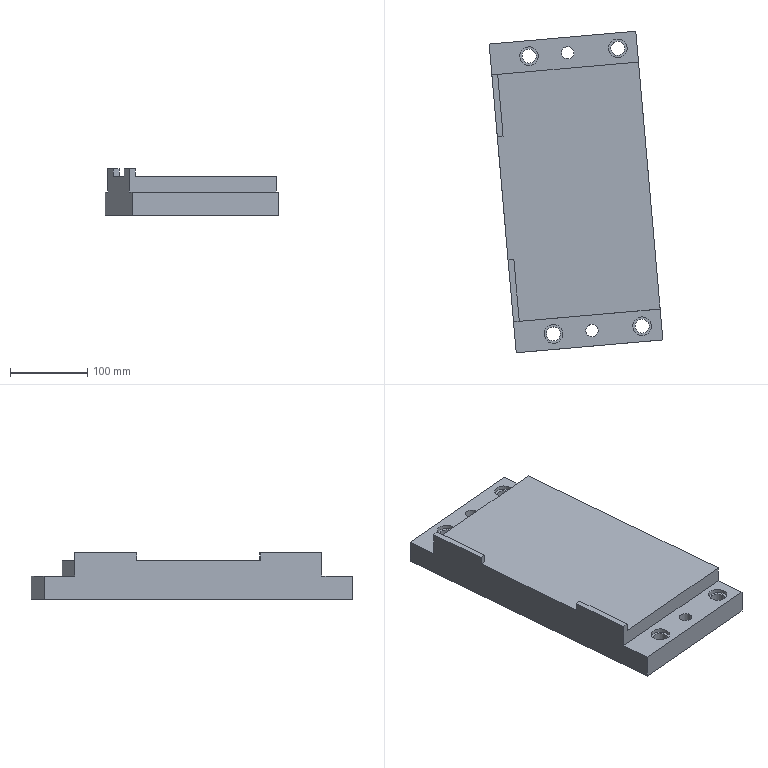Part | NX | features solid 2 | 1 solid | 35 faces | box 224.139 x 415.037 x 60 mm | volume 3448776 mm3 | plane 23 | cylinder 12 | commonest cylinder face diameters 18 x4 24 x4 16 x2 33.267 x2
STEP:
#1=CARTESIAN_POINT('',(824.667,699.536,-260.));
#2=VERTEX_POINT('',#1);
#3=CARTESIAN_POINT('',(831.64,619.841,-260.));
#4=VERTEX_POINT('',#3);
#5=CARTESIAN_POINT('',(824.667,699.536,-260.));
#6=DIRECTION('',(0.08716,-0.9962,0.));
#7=VECTOR('',#6,1000.);
#8=LINE('',#5,#7);
#9=EDGE_CURVE('',#2,#4,#8,.T.);
#10=ORIENTED_EDGE('',*,*,#9,.F.);
#11=CARTESIAN_POINT('',(817.198,698.883,-260.));
#12=VERTEX_POINT('',#11);
#13=CARTESIAN_POINT('',(824.667,699.536,-260.));
#14=DIRECTION('',(-0.9962,-0.08716,0.));
#15=VECTOR('',#14,1000.);
#16=LINE('',#13,#15);
#17=EDGE_CURVE('',#2,#12,#16,.T.);
#18=ORIENTED_EDGE('',*,*,#17,.T.);
#19=CARTESIAN_POINT('',(824.17,619.187,-260.));
#20=VERTEX_POINT('',#19);
#21=CARTESIAN_POINT('',(817.198,698.883,-260.));
#22=DIRECTION('',(0.08716,-0.9962,0.));
#23=VECTOR('',#22,1000.);
#24=LINE('',#21,#23);
#25=EDGE_CURVE('',#12,#20,#24,.T.);
#26=ORIENTED_EDGE('',*,*,#25,.T.);
#27=CARTESIAN_POINT('',(831.64,619.841,-260.));
#28=DIRECTION('',(-0.9962,-0.08716,0.));
#29=VECTOR('',#28,1000.);
#30=LINE('',#27,#29);
#31=EDGE_CURVE('',#4,#20,#30,.T.);
#32=ORIENTED_EDGE('',*,*,#31,.F.);
#33=EDGE_LOOP('',(#10,#18,#26,#32));
#34=FACE_BOUND('',#33,.T.);
#35=CARTESIAN_POINT('',(824.667,699.536,-260.));
#36=DIRECTION('',(0.,0.,-1.));
#37=DIRECTION('',(0.9962,0.08716,0.));
#38=AXIS2_PLACEMENT_3D('',#35,#36,#37);
#39=PLANE('',#38);
#40=ADVANCED_FACE('',(#34),#39,.F.);
#41=CARTESIAN_POINT('',(824.667,699.536,-270.));
#42=VERTEX_POINT('',#41);
#43=CARTESIAN_POINT('',(831.64,619.841,-270.));
#44=VERTEX_POINT('',#43);
#45=CARTESIAN_POINT('',(824.667,699.536,-270.));
#46=DIRECTION('',(0.08716,-0.9962,0.));
#47=VECTOR('',#46,1000.);
#48=LINE('',#45,#47);
#49=EDGE_CURVE('',#42,#44,#48,.T.);
#50=ORIENTED_EDGE('',*,*,#49,.F.);
#51=CARTESIAN_POINT('',(824.667,699.536,-270.));
#52=DIRECTION('',(0.,0.,1.));
#53=VECTOR('',#52,1000.);
#54=LINE('',#51,#53);
#55=EDGE_CURVE('',#42,#2,#54,.T.);
#56=ORIENTED_EDGE('',*,*,#55,.T.);
#57=ORIENTED_EDGE('',*,*,#9,.T.);
#58=CARTESIAN_POINT('',(831.64,619.841,-270.));
#59=DIRECTION('',(0.,0.,1.));
#60=VECTOR('',#59,1000.);
#61=LINE('',#58,#60);
#62=EDGE_CURVE('',#44,#4,#61,.T.);
#63=ORIENTED_EDGE('',*,*,#62,.F.);
#64=EDGE_LOOP('',(#50,#56,#57,#63));
#65=FACE_BOUND('',#64,.T.);
#66=CARTESIAN_POINT('',(824.667,699.536,-270.));
#67=DIRECTION('',(-0.9962,-0.08716,0.));
#68=DIRECTION('',(0.,0.,-1.));
#69=AXIS2_PLACEMENT_3D('',#66,#67,#68);
#70=PLANE('',#69);
#71=ADVANCED_FACE('',(#65),#70,.F.);
#72=CARTESIAN_POINT('',(1006.475,715.443,-290.));
#73=VERTEX_POINT('',#72);
#74=CARTESIAN_POINT('',(817.198,698.883,-290.));
#75=VERTEX_POINT('',#74);
#76=CARTESIAN_POINT('',(1006.475,715.443,-290.));
#77=DIRECTION('',(0.9962,0.08716,0.));
#78=VECTOR('',#77,1000.);
#79=LINE('',#76,#78);
#80=EDGE_CURVE('',#73,#75,#79,.F.);
#81=ORIENTED_EDGE('',*,*,#80,.T.);
#82=CARTESIAN_POINT('',(817.198,698.883,-260.));
#83=DIRECTION('',(0.,0.,-1.));
#84=VECTOR('',#83,1000.);
#85=LINE('',#82,#84);
#86=EDGE_CURVE('',#12,#75,#85,.T.);
#87=ORIENTED_EDGE('',*,*,#86,.F.);
#88=ORIENTED_EDGE('',*,*,#17,.F.);
#89=ORIENTED_EDGE('',*,*,#55,.F.);
#90=CARTESIAN_POINT('',(1006.475,715.443,-270.));
#91=VERTEX_POINT('',#90);
#92=CARTESIAN_POINT('',(1006.475,715.443,-270.));
#93=DIRECTION('',(-0.9962,-0.08716,0.));
#94=VECTOR('',#93,1000.);
#95=LINE('',#92,#94);
#96=EDGE_CURVE('',#91,#42,#95,.T.);
#97=ORIENTED_EDGE('',*,*,#96,.F.);
#98=CARTESIAN_POINT('',(1006.475,715.443,-320.));
#99=DIRECTION('',(0.,0.,1.));
#100=VECTOR('',#99,1000.);
#101=LINE('',#98,#100);
#102=EDGE_CURVE('',#73,#91,#101,.T.);
#103=ORIENTED_EDGE('',*,*,#102,.F.);
#104=EDGE_LOOP('',(#81,#87,#88,#89,#97,#103));
#105=FACE_BOUND('',#104,.T.);
#106=CARTESIAN_POINT('',(1006.475,715.443,-320.));
#107=DIRECTION('',(0.08716,-0.9962,0.));
#108=DIRECTION('',(0.,0.,-1.));
#109=AXIS2_PLACEMENT_3D('',#106,#107,#108);
#110=PLANE('',#109);
#111=ADVANCED_FACE('',(#105),#110,.F.);
#112=CARTESIAN_POINT('',(1034.365,396.66,-290.));
#113=VERTEX_POINT('',#112);
#114=CARTESIAN_POINT('',(1034.365,396.66,-270.));
#115=VERTEX_POINT('',#114);
#116=CARTESIAN_POINT('',(1034.365,396.66,-320.));
#117=DIRECTION('',(0.,0.,1.));
#118=VECTOR('',#117,1000.);
#119=LINE('',#116,#118);
#120=EDGE_CURVE('',#113,#115,#119,.T.);
#121=ORIENTED_EDGE('',*,*,#120,.T.);
#122=CARTESIAN_POINT('',(852.557,380.754,-270.));
#123=VERTEX_POINT('',#122);
#124=CARTESIAN_POINT('',(1034.365,396.66,-270.));
#125=DIRECTION('',(-0.9962,-0.08716,0.));
#126=VECTOR('',#125,1000.);
#127=LINE('',#124,#126);
#128=EDGE_CURVE('',#115,#123,#127,.T.);
#129=ORIENTED_EDGE('',*,*,#128,.T.);
#130=CARTESIAN_POINT('',(852.557,380.754,-260.));
#131=VERTEX_POINT('',#130);
#132=CARTESIAN_POINT('',(852.557,380.754,-270.));
#133=DIRECTION('',(0.,0.,1.));
#134=VECTOR('',#133,1000.);
#135=LINE('',#132,#134);
#136=EDGE_CURVE('',#123,#131,#135,.T.);
#137=ORIENTED_EDGE('',*,*,#136,.T.);
#138=CARTESIAN_POINT('',(845.088,380.101,-260.));
#139=VERTEX_POINT('',#138);
#140=CARTESIAN_POINT('',(852.557,380.754,-260.));
#141=DIRECTION('',(-0.9962,-0.08716,0.));
#142=VECTOR('',#141,1000.);
#143=LINE('',#140,#142);
#144=EDGE_CURVE('',#131,#139,#143,.T.);
#145=ORIENTED_EDGE('',*,*,#144,.T.);
#146=CARTESIAN_POINT('',(845.088,380.101,-290.));
#147=VERTEX_POINT('',#146);
#148=CARTESIAN_POINT('',(845.088,380.101,-260.));
#149=DIRECTION('',(0.,0.,-1.));
#150=VECTOR('',#149,1000.);
#151=LINE('',#148,#150);
#152=EDGE_CURVE('',#139,#147,#151,.T.);
#153=ORIENTED_EDGE('',*,*,#152,.T.);
#154=CARTESIAN_POINT('',(1034.365,396.66,-290.));
#155=DIRECTION('',(0.9962,0.08716,0.));
#156=VECTOR('',#155,1000.);
#157=LINE('',#154,#156);
#158=EDGE_CURVE('',#113,#147,#157,.F.);
#159=ORIENTED_EDGE('',*,*,#158,.F.);
#160=EDGE_LOOP('',(#121,#129,#137,#145,#153,#159));
#161=FACE_BOUND('',#160,.T.);
#162=CARTESIAN_POINT('',(1034.365,396.66,-320.));
#163=DIRECTION('',(0.08716,-0.9962,0.));
#164=DIRECTION('',(0.,0.,-1.));
#165=AXIS2_PLACEMENT_3D('',#162,#163,#164);
#166=PLANE('',#165);
#167=ADVANCED_FACE('',(#161),#166,.T.);
#168=CARTESIAN_POINT('',(923.044,728.22,-320.));
#169=VERTEX_POINT('',#168);
#170=CARTESIAN_POINT('',(915.074,727.522,-320.));
#171=DIRECTION('',(0.,0.,1.));
#172=DIRECTION('',(0.9962,0.08716,0.));
#173=AXIS2_PLACEMENT_3D('',#170,#171,#172);
#174=CIRCLE('',#173,8.);
#175=EDGE_CURVE('',#169,#169,#174,.T.);
#176=ORIENTED_EDGE('',*,*,#175,.T.);
#177=EDGE_LOOP('',(#176));
#178=FACE_BOUND('',#177,.T.);
#179=CARTESIAN_POINT('',(954.42,369.59,-320.));
#180=VERTEX_POINT('',#179);
#181=CARTESIAN_POINT('',(946.45,368.892,-320.));
#182=DIRECTION('',(0.,0.,1.));
#183=DIRECTION('',(0.9962,0.08716,0.));
#184=AXIS2_PLACEMENT_3D('',#181,#182,#183);
#185=CIRCLE('',#184,8.);
#186=EDGE_CURVE('',#180,#180,#185,.T.);
#187=ORIENTED_EDGE('',*,*,#186,.T.);
#188=EDGE_LOOP('',(#187));
#189=FACE_BOUND('',#188,.T.);
#190=CARTESIAN_POINT('',(957.117,533.816,-320.));
#191=VERTEX_POINT('',#190);
#192=CARTESIAN_POINT('',(954.218,566.956,-320.));
#193=VERTEX_POINT('',#192);
#194=CARTESIAN_POINT('',(955.667,550.386,-320.));
#195=DIRECTION('',(0.,0.,1.));
#196=DIRECTION('',(-0.9962,-0.08716,0.));
#197=AXIS2_PLACEMENT_3D('',#194,#195,#196);
#198=CIRCLE('',#197,16.633);
#199=EDGE_CURVE('',#191,#193,#198,.T.);
#200=ORIENTED_EDGE('',*,*,#199,.T.);
#201=CARTESIAN_POINT('',(904.408,562.598,-320.));
#202=VERTEX_POINT('',#201);
#203=CARTESIAN_POINT('',(904.408,562.598,-320.));
#204=DIRECTION('',(0.9962,0.08716,0.));
#205=VECTOR('',#204,1000.);
#206=LINE('',#203,#205);
#207=EDGE_CURVE('',#202,#193,#206,.T.);
#208=ORIENTED_EDGE('',*,*,#207,.F.);
#209=CARTESIAN_POINT('',(907.307,529.459,-320.));
#210=VERTEX_POINT('',#209);
#211=CARTESIAN_POINT('',(905.858,546.028,-320.));
#212=DIRECTION('',(0.,0.,1.));
#213=DIRECTION('',(-0.9962,-0.08716,0.));
#214=AXIS2_PLACEMENT_3D('',#211,#212,#213);
#215=CIRCLE('',#214,16.633);
#216=EDGE_CURVE('',#202,#210,#215,.T.);
#217=ORIENTED_EDGE('',*,*,#216,.T.);
#218=CARTESIAN_POINT('',(957.117,533.816,-320.));
#219=DIRECTION('',(-0.9962,-0.08716,0.));
#220=VECTOR('',#219,1000.);
#221=LINE('',#218,#220);
#222=EDGE_CURVE('',#191,#210,#221,.T.);
#223=ORIENTED_EDGE('',*,*,#222,.F.);
#224=EDGE_LOOP('',(#200,#208,#217,#223));
#225=FACE_BOUND('',#224,.T.);
#226=CARTESIAN_POINT('',(874.23,723.949,-320.));
#227=VERTEX_POINT('',#226);
#228=CARTESIAN_POINT('',(865.265,723.165,-320.));
#229=DIRECTION('',(0.,0.,-1.));
#230=DIRECTION('',(0.9962,0.08716,0.));
#231=AXIS2_PLACEMENT_3D('',#228,#229,#230);
#232=CIRCLE('',#231,9.);
#233=EDGE_CURVE('',#227,#227,#232,.T.);
#234=ORIENTED_EDGE('',*,*,#233,.F.);
#235=EDGE_LOOP('',(#234));
#236=FACE_BOUND('',#235,.T.);
#237=CARTESIAN_POINT('',(988.793,733.972,-320.));
#238=VERTEX_POINT('',#237);
#239=CARTESIAN_POINT('',(979.827,733.188,-320.));
#240=DIRECTION('',(0.,0.,-1.));
#241=DIRECTION('',(0.9962,0.08716,0.));
#242=AXIS2_PLACEMENT_3D('',#239,#240,#241);
#243=CIRCLE('',#242,9.);
#244=EDGE_CURVE('',#238,#238,#243,.T.);
#245=ORIENTED_EDGE('',*,*,#244,.F.);
#246=EDGE_LOOP('',(#245));
#247=FACE_BOUND('',#246,.T.);
#248=CARTESIAN_POINT('',(905.606,365.319,-320.));
#249=VERTEX_POINT('',#248);
#250=CARTESIAN_POINT('',(896.641,364.535,-320.));
#251=DIRECTION('',(0.,0.,1.));
#252=DIRECTION('',(0.9962,0.08716,0.));
#253=AXIS2_PLACEMENT_3D('',#250,#251,#252);
#254=CIRCLE('',#253,9.);
#255=EDGE_CURVE('',#249,#249,#254,.T.);
#256=ORIENTED_EDGE('',*,*,#255,.T.);
#257=EDGE_LOOP('',(#256));
#258=FACE_BOUND('',#257,.T.);
#259=CARTESIAN_POINT('',(1020.169,375.342,-320.));
#260=VERTEX_POINT('',#259);
#261=CARTESIAN_POINT('',(1011.203,374.557,-320.));
#262=DIRECTION('',(0.,0.,1.));
#263=DIRECTION('',(0.9962,0.08716,0.));
#264=AXIS2_PLACEMENT_3D('',#261,#262,#263);
#265=CIRCLE('',#264,9.);
#266=EDGE_CURVE('',#260,#260,#265,.T.);
#267=ORIENTED_EDGE('',*,*,#266,.T.);
#268=EDGE_LOOP('',(#267));
#269=FACE_BOUND('',#268,.T.);
#270=CARTESIAN_POINT('',(813.712,738.731,-320.));
#271=VERTEX_POINT('',#270);
#272=CARTESIAN_POINT('',(848.574,340.253,-320.));
#273=VERTEX_POINT('',#272);
#274=CARTESIAN_POINT('',(817.198,698.883,-320.));
#275=DIRECTION('',(0.08716,-0.9962,0.));
#276=VECTOR('',#275,1000.);
#277=LINE('',#274,#276);
#278=EDGE_CURVE('',#271,#273,#277,.T.);
#279=ORIENTED_EDGE('',*,*,#278,.F.);
#280=CARTESIAN_POINT('',(1002.989,755.29,-320.));
#281=VERTEX_POINT('',#280);
#282=CARTESIAN_POINT('',(1002.989,755.29,-320.));
#283=DIRECTION('',(-0.9962,-0.08716,0.));
#284=VECTOR('',#283,1000.);
#285=LINE('',#282,#284);
#286=EDGE_CURVE('',#281,#271,#285,.T.);
#287=ORIENTED_EDGE('',*,*,#286,.F.);
#288=CARTESIAN_POINT('',(1037.851,356.812,-320.));
#289=VERTEX_POINT('',#288);
#290=CARTESIAN_POINT('',(1006.475,715.443,-320.));
#291=DIRECTION('',(0.08716,-0.9962,0.));
#292=VECTOR('',#291,1000.);
#293=LINE('',#290,#292);
#294=EDGE_CURVE('',#281,#289,#293,.T.);
#295=ORIENTED_EDGE('',*,*,#294,.T.);
#296=CARTESIAN_POINT('',(1037.851,356.812,-320.));
#297=DIRECTION('',(-0.9962,-0.08716,0.));
#298=VECTOR('',#297,1000.);
#299=LINE('',#296,#298);
#300=EDGE_CURVE('',#289,#273,#299,.T.);
#301=ORIENTED_EDGE('',*,*,#300,.T.);
#302=EDGE_LOOP('',(#279,#287,#295,#301));
#303=FACE_BOUND('',#302,.T.);
#304=CARTESIAN_POINT('',(1006.475,715.443,-320.));
#305=DIRECTION('',(0.,0.,-1.));
#306=DIRECTION('',(0.9962,0.08716,0.));
#307=AXIS2_PLACEMENT_3D('',#304,#305,#306);
#308=PLANE('',#307);
#309=ADVANCED_FACE('',(#178,#189,#225,#236,#247,#258,#269,#303),#308,.T.);
#310=ORIENTED_EDGE('',*,*,#25,.F.);
#311=ORIENTED_EDGE('',*,*,#86,.T.);
#312=CARTESIAN_POINT('',(813.712,738.731,-290.));
#313=VERTEX_POINT('',#312);
#314=CARTESIAN_POINT('',(817.198,698.883,-290.));
#315=DIRECTION('',(0.08716,-0.9962,0.));
#316=VECTOR('',#315,1000.);
#317=LINE('',#314,#316);
#318=EDGE_CURVE('',#75,#313,#317,.F.);
#319=ORIENTED_EDGE('',*,*,#318,.T.);
#320=CARTESIAN_POINT('',(813.712,738.731,-320.));
#321=DIRECTION('',(0.,0.,1.));
#322=VECTOR('',#321,1000.);
#323=LINE('',#320,#322);
#324=EDGE_CURVE('',#271,#313,#323,.T.);
#325=ORIENTED_EDGE('',*,*,#324,.F.);
#326=ORIENTED_EDGE('',*,*,#278,.T.);
#327=CARTESIAN_POINT('',(848.574,340.253,-290.));
#328=VERTEX_POINT('',#327);
#329=CARTESIAN_POINT('',(848.574,340.253,-320.));
#330=DIRECTION('',(0.,0.,1.));
#331=VECTOR('',#330,1000.);
#332=LINE('',#329,#331);
#333=EDGE_CURVE('',#273,#328,#332,.T.);
#334=ORIENTED_EDGE('',*,*,#333,.T.);
#335=CARTESIAN_POINT('',(845.088,380.101,-290.));
#336=DIRECTION('',(-0.08716,0.9962,0.));
#337=VECTOR('',#336,1000.);
#338=LINE('',#335,#337);
#339=EDGE_CURVE('',#147,#328,#338,.F.);
#340=ORIENTED_EDGE('',*,*,#339,.F.);
#341=ORIENTED_EDGE('',*,*,#152,.F.);
#342=CARTESIAN_POINT('',(838.115,459.796,-260.));
#343=VERTEX_POINT('',#342);
#344=CARTESIAN_POINT('',(817.198,698.883,-260.));
#345=DIRECTION('',(0.08716,-0.9962,0.));
#346=VECTOR('',#345,1000.);
#347=LINE('',#344,#346);
#348=EDGE_CURVE('',#343,#139,#347,.T.);
#349=ORIENTED_EDGE('',*,*,#348,.F.);
#350=CARTESIAN_POINT('',(838.115,459.796,-270.));
#351=VERTEX_POINT('',#350);
#352=CARTESIAN_POINT('',(838.115,459.796,-260.));
#353=DIRECTION('',(0.,0.,-1.));
#354=VECTOR('',#353,1000.);
#355=LINE('',#352,#354);
#356=EDGE_CURVE('',#351,#343,#355,.F.);
#357=ORIENTED_EDGE('',*,*,#356,.F.);
#358=CARTESIAN_POINT('',(824.17,619.187,-270.));
#359=VERTEX_POINT('',#358);
#360=CARTESIAN_POINT('',(817.198,698.883,-270.));
#361=DIRECTION('',(-0.08716,0.9962,0.));
#362=VECTOR('',#361,1000.);
#363=LINE('',#360,#362);
#364=EDGE_CURVE('',#359,#351,#363,.F.);
#365=ORIENTED_EDGE('',*,*,#364,.F.);
#366=CARTESIAN_POINT('',(824.17,619.187,-260.));
#367=DIRECTION('',(0.,0.,-1.));
#368=VECTOR('',#367,1000.);
#369=LINE('',#366,#368);
#370=EDGE_CURVE('',#20,#359,#369,.T.);
#371=ORIENTED_EDGE('',*,*,#370,.F.);
#372=EDGE_LOOP('',(#310,#311,#319,#325,#326,#334,#340,#341,#349,#357,#365,#371));
#373=FACE_BOUND('',#372,.T.);
#374=CARTESIAN_POINT('',(817.198,698.883,-260.));
#375=DIRECTION('',(0.9962,0.08716,0.));
#376=DIRECTION('',(0.,0.,1.));
#377=AXIS2_PLACEMENT_3D('',#374,#375,#376);
#378=PLANE('',#377);
#379=ADVANCED_FACE('',(#373),#378,.F.);
#380=ORIENTED_EDGE('',*,*,#348,.T.);
#381=ORIENTED_EDGE('',*,*,#144,.F.);
#382=CARTESIAN_POINT('',(845.585,460.45,-260.));
#383=VERTEX_POINT('',#382);
#384=CARTESIAN_POINT('',(824.667,699.536,-260.));
#385=DIRECTION('',(0.08716,-0.9962,0.));
#386=VECTOR('',#385,1000.);
#387=LINE('',#384,#386);
#388=EDGE_CURVE('',#383,#131,#387,.T.);
#389=ORIENTED_EDGE('',*,*,#388,.F.);
#390=CARTESIAN_POINT('',(845.585,460.45,-260.));
#391=DIRECTION('',(-0.9962,-0.08716,0.));
#392=VECTOR('',#391,1000.);
#393=LINE('',#390,#392);
#394=EDGE_CURVE('',#343,#383,#393,.F.);
#395=ORIENTED_EDGE('',*,*,#394,.F.);
#396=EDGE_LOOP('',(#380,#381,#389,#395));
#397=FACE_BOUND('',#396,.T.);
#398=CARTESIAN_POINT('',(824.667,699.536,-260.));
#399=DIRECTION('',(0.,0.,-1.));
#400=DIRECTION('',(0.9962,0.08716,0.));
#401=AXIS2_PLACEMENT_3D('',#398,#399,#400);
#402=PLANE('',#401);
#403=ADVANCED_FACE('',(#397),#402,.F.);
#404=ORIENTED_EDGE('',*,*,#388,.T.);
#405=ORIENTED_EDGE('',*,*,#136,.F.);
#406=CARTESIAN_POINT('',(845.585,460.45,-270.));
#407=VERTEX_POINT('',#406);
#408=CARTESIAN_POINT('',(824.667,699.536,-270.));
#409=DIRECTION('',(0.08716,-0.9962,0.));
#410=VECTOR('',#409,1000.);
#411=LINE('',#408,#410);
#412=EDGE_CURVE('',#407,#123,#411,.T.);
#413=ORIENTED_EDGE('',*,*,#412,.F.);
#414=CARTESIAN_POINT('',(845.585,460.45,-270.));
#415=DIRECTION('',(0.,0.,1.));
#416=VECTOR('',#415,1000.);
#417=LINE('',#414,#416);
#418=EDGE_CURVE('',#407,#383,#417,.T.);
#419=ORIENTED_EDGE('',*,*,#418,.T.);
#420=EDGE_LOOP('',(#404,#405,#413,#419));
#421=FACE_BOUND('',#420,.T.);
#422=CARTESIAN_POINT('',(824.667,699.536,-270.));
#423=DIRECTION('',(-0.9962,-0.08716,0.));
#424=DIRECTION('',(0.,0.,-1.));
#425=AXIS2_PLACEMENT_3D('',#422,#423,#424);
#426=PLANE('',#425);
#427=ADVANCED_FACE('',(#421),#426,.F.);
#428=ORIENTED_EDGE('',*,*,#128,.F.);
#429=CARTESIAN_POINT('',(1006.475,715.443,-270.));
#430=DIRECTION('',(0.08716,-0.9962,0.));
#431=VECTOR('',#430,1000.);
#432=LINE('',#429,#431);
#433=EDGE_CURVE('',#91,#115,#432,.T.);
#434=ORIENTED_EDGE('',*,*,#433,.F.);
#435=ORIENTED_EDGE('',*,*,#96,.T.);
#436=ORIENTED_EDGE('',*,*,#49,.T.);
#437=CARTESIAN_POINT('',(831.64,619.841,-270.));
#438=DIRECTION('',(-0.9962,-0.08716,0.));
#439=VECTOR('',#438,1000.);
#440=LINE('',#437,#439);
#441=EDGE_CURVE('',#44,#359,#440,.T.);
#442=ORIENTED_EDGE('',*,*,#441,.T.);
#443=ORIENTED_EDGE('',*,*,#364,.T.);
#444=CARTESIAN_POINT('',(845.585,460.45,-270.));
#445=DIRECTION('',(-0.9962,-0.08716,0.));
#446=VECTOR('',#445,1000.);
#447=LINE('',#444,#446);
#448=EDGE_CURVE('',#407,#351,#447,.T.);
#449=ORIENTED_EDGE('',*,*,#448,.F.);
#450=ORIENTED_EDGE('',*,*,#412,.T.);
#451=EDGE_LOOP('',(#428,#434,#435,#436,#442,#443,#449,#450));
#452=FACE_BOUND('',#451,.T.);
#453=CARTESIAN_POINT('',(1006.475,715.443,-270.));
#454=DIRECTION('',(0.,0.,-1.));
#455=DIRECTION('',(0.9962,0.08716,0.));
#456=AXIS2_PLACEMENT_3D('',#453,#454,#455);
#457=PLANE('',#456);
#458=ADVANCED_FACE('',(#452),#457,.F.);
#459=ORIENTED_EDGE('',*,*,#294,.F.);
#460=CARTESIAN_POINT('',(1002.989,755.29,-290.));
#461=VERTEX_POINT('',#460);
#462=CARTESIAN_POINT('',(1002.989,755.29,-320.));
#463=DIRECTION('',(0.,0.,1.));
#464=VECTOR('',#463,1000.);
#465=LINE('',#462,#464);
#466=EDGE_CURVE('',#281,#461,#465,.T.);
#467=ORIENTED_EDGE('',*,*,#466,.T.);
#468=CARTESIAN_POINT('',(1006.475,715.443,-290.));
#469=DIRECTION('',(0.08716,-0.9962,0.));
#470=VECTOR('',#469,1000.);
#471=LINE('',#468,#470);
#472=EDGE_CURVE('',#73,#461,#471,.F.);
#473=ORIENTED_EDGE('',*,*,#472,.F.);
#474=ORIENTED_EDGE('',*,*,#102,.T.);
#475=ORIENTED_EDGE('',*,*,#433,.T.);
#476=ORIENTED_EDGE('',*,*,#120,.F.);
#477=CARTESIAN_POINT('',(1037.851,356.812,-290.));
#478=VERTEX_POINT('',#477);
#479=CARTESIAN_POINT('',(1034.365,396.66,-290.));
#480=DIRECTION('',(-0.08716,0.9962,0.));
#481=VECTOR('',#480,1000.);
#482=LINE('',#479,#481);
#483=EDGE_CURVE('',#113,#478,#482,.F.);
#484=ORIENTED_EDGE('',*,*,#483,.T.);
#485=CARTESIAN_POINT('',(1037.851,356.812,-320.));
#486=DIRECTION('',(0.,0.,1.));
#487=VECTOR('',#486,1000.);
#488=LINE('',#485,#487);
#489=EDGE_CURVE('',#289,#478,#488,.T.);
#490=ORIENTED_EDGE('',*,*,#489,.F.);
#491=EDGE_LOOP('',(#459,#467,#473,#474,#475,#476,#484,#490));
#492=FACE_BOUND('',#491,.T.);
#493=CARTESIAN_POINT('',(1006.475,715.443,-320.));
#494=DIRECTION('',(-0.9962,-0.08716,0.));
#495=DIRECTION('',(0.,0.,-1.));
#496=AXIS2_PLACEMENT_3D('',#493,#494,#495);
#497=PLANE('',#496);
#498=ADVANCED_FACE('',(#492),#497,.F.);
#499=ORIENTED_EDGE('',*,*,#489,.T.);
#500=CARTESIAN_POINT('',(1037.851,356.812,-290.));
#501=DIRECTION('',(0.9962,0.08716,0.));
#502=VECTOR('',#501,1000.);
#503=LINE('',#500,#502);
#504=EDGE_CURVE('',#478,#328,#503,.F.);
#505=ORIENTED_EDGE('',*,*,#504,.T.);
#506=ORIENTED_EDGE('',*,*,#333,.F.);
#507=ORIENTED_EDGE('',*,*,#300,.F.);
#508=EDGE_LOOP('',(#499,#505,#506,#507));
#509=FACE_BOUND('',#508,.T.);
#510=CARTESIAN_POINT('',(1037.851,356.812,-320.));
#511=DIRECTION('',(-0.08716,0.9962,0.));
#512=DIRECTION('',(-0.9962,-0.08716,0.));
#513=AXIS2_PLACEMENT_3D('',#510,#511,#512);
#514=PLANE('',#513);
#515=ADVANCED_FACE('',(#509),#514,.F.);
#516=CARTESIAN_POINT('',(954.42,369.59,-290.));
#517=VERTEX_POINT('',#516);
#518=CARTESIAN_POINT('',(946.45,368.892,-290.));
#519=DIRECTION('',(0.,0.,1.));
#520=DIRECTION('',(0.9962,0.08716,0.));
#521=AXIS2_PLACEMENT_3D('',#518,#519,#520);
#522=CIRCLE('',#521,8.);
#523=EDGE_CURVE('',#517,#517,#522,.T.);
#524=ORIENTED_EDGE('',*,*,#523,.F.);
#525=EDGE_LOOP('',(#524));
#526=FACE_BOUND('',#525,.T.);
#527=CARTESIAN_POINT('',(908.595,365.58,-290.));
#528=VERTEX_POINT('',#527);
#529=CARTESIAN_POINT('',(896.641,364.535,-290.));
#530=DIRECTION('',(0.,0.,1.));
#531=DIRECTION('',(0.9962,0.08716,0.));
#532=AXIS2_PLACEMENT_3D('',#529,#530,#531);
#533=CIRCLE('',#532,12.);
#534=EDGE_CURVE('',#528,#528,#533,.T.);
#535=ORIENTED_EDGE('',*,*,#534,.F.);
#536=EDGE_LOOP('',(#535));
#537=FACE_BOUND('',#536,.T.);
#538=CARTESIAN_POINT('',(1023.157,375.603,-290.));
#539=VERTEX_POINT('',#538);
#540=CARTESIAN_POINT('',(1011.203,374.557,-290.));
#541=DIRECTION('',(0.,0.,1.));
#542=DIRECTION('',(0.9962,0.08716,0.));
#543=AXIS2_PLACEMENT_3D('',#540,#541,#542);
#544=CIRCLE('',#543,12.);
#545=EDGE_CURVE('',#539,#539,#544,.T.);
#546=ORIENTED_EDGE('',*,*,#545,.F.);
#547=EDGE_LOOP('',(#546));
#548=FACE_BOUND('',#547,.T.);
#549=ORIENTED_EDGE('',*,*,#504,.F.);
#550=ORIENTED_EDGE('',*,*,#483,.F.);
#551=ORIENTED_EDGE('',*,*,#158,.T.);
#552=ORIENTED_EDGE('',*,*,#339,.T.);
#553=EDGE_LOOP('',(#549,#550,#551,#552));
#554=FACE_BOUND('',#553,.T.);
#555=CARTESIAN_POINT('',(1034.365,396.66,-290.));
#556=DIRECTION('',(0.,0.,-1.));
#557=DIRECTION('',(0.9962,0.08716,0.));
#558=AXIS2_PLACEMENT_3D('',#555,#556,#557);
#559=PLANE('',#558);
#560=ADVANCED_FACE('',(#526,#537,#548,#554),#559,.F.);
#561=ORIENTED_EDGE('',*,*,#466,.F.);
#562=ORIENTED_EDGE('',*,*,#286,.T.);
#563=ORIENTED_EDGE('',*,*,#324,.T.);
#564=CARTESIAN_POINT('',(1002.989,755.29,-290.));
#565=DIRECTION('',(0.9962,0.08716,0.));
#566=VECTOR('',#565,1000.);
#567=LINE('',#564,#566);
#568=EDGE_CURVE('',#461,#313,#567,.F.);
#569=ORIENTED_EDGE('',*,*,#568,.F.);
#570=EDGE_LOOP('',(#561,#562,#563,#569));
#571=FACE_BOUND('',#570,.T.);
#572=CARTESIAN_POINT('',(1002.989,755.29,-320.));
#573=DIRECTION('',(0.08716,-0.9962,0.));
#574=DIRECTION('',(-0.9962,-0.08716,0.));
#575=AXIS2_PLACEMENT_3D('',#572,#573,#574);
#576=PLANE('',#575);
#577=ADVANCED_FACE('',(#571),#576,.F.);
#578=CARTESIAN_POINT('',(923.044,728.22,-290.));
#579=VERTEX_POINT('',#578);
#580=CARTESIAN_POINT('',(915.074,727.522,-290.));
#581=DIRECTION('',(0.,0.,1.));
#582=DIRECTION('',(0.9962,0.08716,0.));
#583=AXIS2_PLACEMENT_3D('',#580,#581,#582);
#584=CIRCLE('',#583,8.);
#585=EDGE_CURVE('',#579,#579,#584,.T.);
#586=ORIENTED_EDGE('',*,*,#585,.F.);
#587=EDGE_LOOP('',(#586));
#588=FACE_BOUND('',#587,.T.);
#589=CARTESIAN_POINT('',(877.219,724.211,-290.));
#590=VERTEX_POINT('',#589);
#591=CARTESIAN_POINT('',(865.265,723.165,-290.));
#592=DIRECTION('',(0.,0.,-1.));
#593=DIRECTION('',(0.9962,0.08716,0.));
#594=AXIS2_PLACEMENT_3D('',#591,#592,#593);
#595=CIRCLE('',#594,12.);
#596=EDGE_CURVE('',#590,#590,#595,.T.);
#597=ORIENTED_EDGE('',*,*,#596,.T.);
#598=EDGE_LOOP('',(#597));
#599=FACE_BOUND('',#598,.T.);
#600=CARTESIAN_POINT('',(991.781,734.233,-290.));
#601=VERTEX_POINT('',#600);
#602=CARTESIAN_POINT('',(979.827,733.188,-290.));
#603=DIRECTION('',(0.,0.,-1.));
#604=DIRECTION('',(0.9962,0.08716,0.));
#605=AXIS2_PLACEMENT_3D('',#602,#603,#604);
#606=CIRCLE('',#605,12.);
#607=EDGE_CURVE('',#601,#601,#606,.T.);
#608=ORIENTED_EDGE('',*,*,#607,.T.);
#609=EDGE_LOOP('',(#608));
#610=FACE_BOUND('',#609,.T.);
#611=ORIENTED_EDGE('',*,*,#568,.T.);
#612=ORIENTED_EDGE('',*,*,#318,.F.);
#613=ORIENTED_EDGE('',*,*,#80,.F.);
#614=ORIENTED_EDGE('',*,*,#472,.T.);
#615=EDGE_LOOP('',(#611,#612,#613,#614));
#616=FACE_BOUND('',#615,.T.);
#617=CARTESIAN_POINT('',(1006.475,715.443,-290.));
#618=DIRECTION('',(0.,0.,-1.));
#619=DIRECTION('',(0.9962,0.08716,0.));
#620=AXIS2_PLACEMENT_3D('',#617,#618,#619);
#621=PLANE('',#620);
#622=ADVANCED_FACE('',(#588,#599,#610,#616),#621,.F.);
#623=ORIENTED_EDGE('',*,*,#31,.T.);
#624=ORIENTED_EDGE('',*,*,#370,.T.);
#625=ORIENTED_EDGE('',*,*,#441,.F.);
#626=ORIENTED_EDGE('',*,*,#62,.T.);
#627=EDGE_LOOP('',(#623,#624,#625,#626));
#628=FACE_BOUND('',#627,.T.);
#629=CARTESIAN_POINT('',(831.64,619.841,-270.));
#630=DIRECTION('',(-0.08716,0.9962,0.));
#631=DIRECTION('',(0.,0.,1.));
#632=AXIS2_PLACEMENT_3D('',#629,#630,#631);
#633=PLANE('',#632);
#634=ADVANCED_FACE('',(#628),#633,.F.);
#635=ORIENTED_EDGE('',*,*,#448,.T.);
#636=ORIENTED_EDGE('',*,*,#356,.T.);
#637=ORIENTED_EDGE('',*,*,#394,.T.);
#638=ORIENTED_EDGE('',*,*,#418,.F.);
#639=EDGE_LOOP('',(#635,#636,#637,#638));
#640=FACE_BOUND('',#639,.T.);
#641=CARTESIAN_POINT('',(845.585,460.45,-270.));
#642=DIRECTION('',(-0.08716,0.9962,0.));
#643=DIRECTION('',(0.,0.,1.));
#644=AXIS2_PLACEMENT_3D('',#641,#642,#643);
#645=PLANE('',#644);
#646=ADVANCED_FACE('',(#640),#645,.T.);
#647=ORIENTED_EDGE('',*,*,#266,.F.);
#648=EDGE_LOOP('',(#647));
#649=FACE_BOUND('',#648,.T.);
#650=CARTESIAN_POINT('',(1020.169,375.342,-295.));
#651=VERTEX_POINT('',#650);
#652=CARTESIAN_POINT('',(1011.203,374.557,-295.));
#653=DIRECTION('',(0.,0.,1.));
#654=DIRECTION('',(0.9962,0.08716,0.));
#655=AXIS2_PLACEMENT_3D('',#652,#653,#654);
#656=CIRCLE('',#655,9.);
#657=EDGE_CURVE('',#651,#651,#656,.T.);
#658=ORIENTED_EDGE('',*,*,#657,.T.);
#659=EDGE_LOOP('',(#658));
#660=FACE_BOUND('',#659,.T.);
#661=CARTESIAN_POINT('',(1011.203,374.557,-320.));
#662=DIRECTION('',(0.,0.,-1.));
#663=DIRECTION('',(0.9962,0.08716,0.));
#664=AXIS2_PLACEMENT_3D('',#661,#662,#663);
#665=CYLINDRICAL_SURFACE('',#664,9.);
#666=ADVANCED_FACE('',(#649,#660),#665,.F.);
#667=ORIENTED_EDGE('',*,*,#657,.F.);
#668=EDGE_LOOP('',(#667));
#669=FACE_BOUND('',#668,.T.);
#670=CARTESIAN_POINT('',(1023.157,375.603,-295.));
#671=VERTEX_POINT('',#670);
#672=CARTESIAN_POINT('',(1011.203,374.557,-295.));
#673=DIRECTION('',(0.,0.,1.));
#674=DIRECTION('',(0.9962,0.08716,0.));
#675=AXIS2_PLACEMENT_3D('',#672,#673,#674);
#676=CIRCLE('',#675,12.);
#677=EDGE_CURVE('',#671,#671,#676,.T.);
#678=ORIENTED_EDGE('',*,*,#677,.T.);
#679=EDGE_LOOP('',(#678));
#680=FACE_BOUND('',#679,.T.);
#681=CARTESIAN_POINT('',(1011.203,374.557,-295.));
#682=DIRECTION('',(0.,0.,-1.));
#683=DIRECTION('',(0.9962,0.08716,0.));
#684=AXIS2_PLACEMENT_3D('',#681,#682,#683);
#685=PLANE('',#684);
#686=ADVANCED_FACE('',(#669,#680),#685,.F.);
#687=ORIENTED_EDGE('',*,*,#677,.F.);
#688=EDGE_LOOP('',(#687));
#689=FACE_BOUND('',#688,.T.);
#690=ORIENTED_EDGE('',*,*,#545,.T.);
#691=EDGE_LOOP('',(#690));
#692=FACE_BOUND('',#691,.T.);
#693=CARTESIAN_POINT('',(1011.203,374.557,-290.));
#694=DIRECTION('',(0.,0.,-1.));
#695=DIRECTION('',(0.9962,0.08716,0.));
#696=AXIS2_PLACEMENT_3D('',#693,#694,#695);
#697=CYLINDRICAL_SURFACE('',#696,12.);
#698=ADVANCED_FACE('',(#689,#692),#697,.F.);
#699=ORIENTED_EDGE('',*,*,#255,.F.);
#700=EDGE_LOOP('',(#699));
#701=FACE_BOUND('',#700,.T.);
#702=CARTESIAN_POINT('',(905.606,365.319,-295.));
#703=VERTEX_POINT('',#702);
#704=CARTESIAN_POINT('',(896.641,364.535,-295.));
#705=DIRECTION('',(0.,0.,1.));
#706=DIRECTION('',(0.9962,0.08716,0.));
#707=AXIS2_PLACEMENT_3D('',#704,#705,#706);
#708=CIRCLE('',#707,9.);
#709=EDGE_CURVE('',#703,#703,#708,.T.);
#710=ORIENTED_EDGE('',*,*,#709,.T.);
#711=EDGE_LOOP('',(#710));
#712=FACE_BOUND('',#711,.T.);
#713=CARTESIAN_POINT('',(896.641,364.535,-320.));
#714=DIRECTION('',(0.,0.,-1.));
#715=DIRECTION('',(0.9962,0.08716,0.));
#716=AXIS2_PLACEMENT_3D('',#713,#714,#715);
#717=CYLINDRICAL_SURFACE('',#716,9.);
#718=ADVANCED_FACE('',(#701,#712),#717,.F.);
#719=ORIENTED_EDGE('',*,*,#709,.F.);
#720=EDGE_LOOP('',(#719));
#721=FACE_BOUND('',#720,.T.);
#722=CARTESIAN_POINT('',(908.595,365.58,-295.));
#723=VERTEX_POINT('',#722);
#724=CARTESIAN_POINT('',(896.641,364.535,-295.));
#725=DIRECTION('',(0.,0.,1.));
#726=DIRECTION('',(0.9962,0.08716,0.));
#727=AXIS2_PLACEMENT_3D('',#724,#725,#726);
#728=CIRCLE('',#727,12.);
#729=EDGE_CURVE('',#723,#723,#728,.T.);
#730=ORIENTED_EDGE('',*,*,#729,.T.);
#731=EDGE_LOOP('',(#730));
#732=FACE_BOUND('',#731,.T.);
#733=CARTESIAN_POINT('',(871.736,362.356,-295.));
#734=DIRECTION('',(0.,0.,-1.));
#735=DIRECTION('',(0.9962,0.08716,0.));
#736=AXIS2_PLACEMENT_3D('',#733,#734,#735);
#737=PLANE('',#736);
#738=ADVANCED_FACE('',(#721,#732),#737,.F.);
#739=ORIENTED_EDGE('',*,*,#729,.F.);
#740=EDGE_LOOP('',(#739));
#741=FACE_BOUND('',#740,.T.);
#742=ORIENTED_EDGE('',*,*,#534,.T.);
#743=EDGE_LOOP('',(#742));
#744=FACE_BOUND('',#743,.T.);
#745=CARTESIAN_POINT('',(896.641,364.535,-290.));
#746=DIRECTION('',(0.,0.,-1.));
#747=DIRECTION('',(0.9962,0.08716,0.));
#748=AXIS2_PLACEMENT_3D('',#745,#746,#747);
#749=CYLINDRICAL_SURFACE('',#748,12.);
#750=ADVANCED_FACE('',(#741,#744),#749,.F.);
#751=ORIENTED_EDGE('',*,*,#244,.T.);
#752=EDGE_LOOP('',(#751));
#753=FACE_BOUND('',#752,.T.);
#754=CARTESIAN_POINT('',(988.793,733.972,-295.));
#755=VERTEX_POINT('',#754);
#756=CARTESIAN_POINT('',(979.827,733.188,-295.));
#757=DIRECTION('',(0.,0.,-1.));
#758=DIRECTION('',(0.9962,0.08716,0.));
#759=AXIS2_PLACEMENT_3D('',#756,#757,#758);
#760=CIRCLE('',#759,9.);
#761=EDGE_CURVE('',#755,#755,#760,.T.);
#762=ORIENTED_EDGE('',*,*,#761,.F.);
#763=EDGE_LOOP('',(#762));
#764=FACE_BOUND('',#763,.T.);
#765=CARTESIAN_POINT('',(979.827,733.188,-320.));
#766=DIRECTION('',(0.,0.,-1.));
#767=DIRECTION('',(0.9962,0.08716,0.));
#768=AXIS2_PLACEMENT_3D('',#765,#766,#767);
#769=CYLINDRICAL_SURFACE('',#768,9.);
#770=ADVANCED_FACE('',(#753,#764),#769,.F.);
#771=ORIENTED_EDGE('',*,*,#761,.T.);
#772=EDGE_LOOP('',(#771));
#773=FACE_BOUND('',#772,.T.);
#774=CARTESIAN_POINT('',(991.781,734.233,-295.));
#775=VERTEX_POINT('',#774);
#776=CARTESIAN_POINT('',(979.827,733.188,-295.));
#777=DIRECTION('',(0.,0.,-1.));
#778=DIRECTION('',(0.9962,0.08716,0.));
#779=AXIS2_PLACEMENT_3D('',#776,#777,#778);
#780=CIRCLE('',#779,12.);
#781=EDGE_CURVE('',#775,#775,#780,.T.);
#782=ORIENTED_EDGE('',*,*,#781,.F.);
#783=EDGE_LOOP('',(#782));
#784=FACE_BOUND('',#783,.T.);
#785=CARTESIAN_POINT('',(979.827,733.188,-295.));
#786=DIRECTION('',(0.,0.,-1.));
#787=DIRECTION('',(0.9962,0.08716,0.));
#788=AXIS2_PLACEMENT_3D('',#785,#786,#787);
#789=PLANE('',#788);
#790=ADVANCED_FACE('',(#773,#784),#789,.F.);
#791=ORIENTED_EDGE('',*,*,#781,.T.);
#792=EDGE_LOOP('',(#791));
#793=FACE_BOUND('',#792,.T.);
#794=ORIENTED_EDGE('',*,*,#607,.F.);
#795=EDGE_LOOP('',(#794));
#796=FACE_BOUND('',#795,.T.);
#797=CARTESIAN_POINT('',(979.827,733.188,-290.));
#798=DIRECTION('',(0.,0.,-1.));
#799=DIRECTION('',(0.9962,0.08716,0.));
#800=AXIS2_PLACEMENT_3D('',#797,#798,#799);
#801=CYLINDRICAL_SURFACE('',#800,12.);
#802=ADVANCED_FACE('',(#793,#796),#801,.F.);
#803=ORIENTED_EDGE('',*,*,#233,.T.);
#804=EDGE_LOOP('',(#803));
#805=FACE_BOUND('',#804,.T.);
#806=CARTESIAN_POINT('',(874.23,723.949,-295.));
#807=VERTEX_POINT('',#806);
#808=CARTESIAN_POINT('',(865.265,723.165,-295.));
#809=DIRECTION('',(0.,0.,-1.));
#810=DIRECTION('',(0.9962,0.08716,0.));
#811=AXIS2_PLACEMENT_3D('',#808,#809,#810);
#812=CIRCLE('',#811,9.);
#813=EDGE_CURVE('',#807,#807,#812,.T.);
#814=ORIENTED_EDGE('',*,*,#813,.F.);
#815=EDGE_LOOP('',(#814));
#816=FACE_BOUND('',#815,.T.);
#817=CARTESIAN_POINT('',(865.265,723.165,-320.));
#818=DIRECTION('',(0.,0.,-1.));
#819=DIRECTION('',(0.9962,0.08716,0.));
#820=AXIS2_PLACEMENT_3D('',#817,#818,#819);
#821=CYLINDRICAL_SURFACE('',#820,9.);
#822=ADVANCED_FACE('',(#805,#816),#821,.F.);
#823=ORIENTED_EDGE('',*,*,#813,.T.);
#824=EDGE_LOOP('',(#823));
#825=FACE_BOUND('',#824,.T.);
#826=CARTESIAN_POINT('',(877.219,724.211,-295.));
#827=VERTEX_POINT('',#826);
#828=CARTESIAN_POINT('',(865.265,723.165,-295.));
#829=DIRECTION('',(0.,0.,-1.));
#830=DIRECTION('',(0.9962,0.08716,0.));
#831=AXIS2_PLACEMENT_3D('',#828,#829,#830);
#832=CIRCLE('',#831,12.);
#833=EDGE_CURVE('',#827,#827,#832,.T.);
#834=ORIENTED_EDGE('',*,*,#833,.F.);
#835=EDGE_LOOP('',(#834));
#836=FACE_BOUND('',#835,.T.);
#837=CARTESIAN_POINT('',(840.36,720.986,-295.));
#838=DIRECTION('',(0.,0.,-1.));
#839=DIRECTION('',(0.9962,0.08716,0.));
#840=AXIS2_PLACEMENT_3D('',#837,#838,#839);
#841=PLANE('',#840);
#842=ADVANCED_FACE('',(#825,#836),#841,.F.);
#843=ORIENTED_EDGE('',*,*,#833,.T.);
#844=EDGE_LOOP('',(#843));
#845=FACE_BOUND('',#844,.T.);
#846=ORIENTED_EDGE('',*,*,#596,.F.);
#847=EDGE_LOOP('',(#846));
#848=FACE_BOUND('',#847,.T.);
#849=CARTESIAN_POINT('',(865.265,723.165,-290.));
#850=DIRECTION('',(0.,0.,-1.));
#851=DIRECTION('',(0.9962,0.08716,0.));
#852=AXIS2_PLACEMENT_3D('',#849,#850,#851);
#853=CYLINDRICAL_SURFACE('',#852,12.);
#854=ADVANCED_FACE('',(#845,#848),#853,.F.);
#855=ORIENTED_EDGE('',*,*,#199,.F.);
#856=CARTESIAN_POINT('',(957.117,533.816,-315.));
#857=VERTEX_POINT('',#856);
#858=CARTESIAN_POINT('',(957.117,533.816,-315.));
#859=DIRECTION('',(0.,0.,-1.));
#860=VECTOR('',#859,1000.);
#861=LINE('',#858,#860);
#862=EDGE_CURVE('',#857,#191,#861,.T.);
#863=ORIENTED_EDGE('',*,*,#862,.F.);
#864=CARTESIAN_POINT('',(954.218,566.956,-315.));
#865=VERTEX_POINT('',#864);
#866=CARTESIAN_POINT('',(955.667,550.386,-315.));
#867=DIRECTION('',(0.,0.,1.));
#868=DIRECTION('',(-0.9962,-0.08716,0.));
#869=AXIS2_PLACEMENT_3D('',#866,#867,#868);
#870=CIRCLE('',#869,16.633);
#871=EDGE_CURVE('',#857,#865,#870,.T.);
#872=ORIENTED_EDGE('',*,*,#871,.T.);
#873=CARTESIAN_POINT('',(954.218,566.956,-315.));
#874=DIRECTION('',(0.,0.,-1.));
#875=VECTOR('',#874,1000.);
#876=LINE('',#873,#875);
#877=EDGE_CURVE('',#865,#193,#876,.T.);
#878=ORIENTED_EDGE('',*,*,#877,.T.);
#879=EDGE_LOOP('',(#855,#863,#872,#878));
#880=FACE_BOUND('',#879,.T.);
#881=CARTESIAN_POINT('',(955.667,550.386,-315.));
#882=DIRECTION('',(0.,0.,-1.));
#883=DIRECTION('',(0.9962,0.08716,0.));
#884=AXIS2_PLACEMENT_3D('',#881,#882,#883);
#885=CYLINDRICAL_SURFACE('',#884,16.633);
#886=ADVANCED_FACE('',(#880),#885,.F.);
#887=ORIENTED_EDGE('',*,*,#207,.T.);
#888=ORIENTED_EDGE('',*,*,#877,.F.);
#889=CARTESIAN_POINT('',(904.408,562.598,-315.));
#890=VERTEX_POINT('',#889);
#891=CARTESIAN_POINT('',(904.408,562.598,-315.));
#892=DIRECTION('',(0.9962,0.08716,0.));
#893=VECTOR('',#892,1000.);
#894=LINE('',#891,#893);
#895=EDGE_CURVE('',#890,#865,#894,.T.);
#896=ORIENTED_EDGE('',*,*,#895,.F.);
#897=CARTESIAN_POINT('',(904.408,562.598,-315.));
#898=DIRECTION('',(0.,0.,-1.));
#899=VECTOR('',#898,1000.);
#900=LINE('',#897,#899);
#901=EDGE_CURVE('',#890,#202,#900,.T.);
#902=ORIENTED_EDGE('',*,*,#901,.T.);
#903=EDGE_LOOP('',(#887,#888,#896,#902));
#904=FACE_BOUND('',#903,.T.);
#905=CARTESIAN_POINT('',(904.408,562.598,-315.));
#906=DIRECTION('',(0.08716,-0.9962,0.));
#907=DIRECTION('',(-0.9962,-0.08716,0.));
#908=AXIS2_PLACEMENT_3D('',#905,#906,#907);
#909=PLANE('',#908);
#910=ADVANCED_FACE('',(#904),#909,.T.);
#911=ORIENTED_EDGE('',*,*,#216,.F.);
#912=ORIENTED_EDGE('',*,*,#901,.F.);
#913=CARTESIAN_POINT('',(907.307,529.459,-315.));
#914=VERTEX_POINT('',#913);
#915=CARTESIAN_POINT('',(905.858,546.028,-315.));
#916=DIRECTION('',(0.,0.,1.));
#917=DIRECTION('',(-0.9962,-0.08716,0.));
#918=AXIS2_PLACEMENT_3D('',#915,#916,#917);
#919=CIRCLE('',#918,16.633);
#920=EDGE_CURVE('',#890,#914,#919,.T.);
#921=ORIENTED_EDGE('',*,*,#920,.T.);
#922=CARTESIAN_POINT('',(907.307,529.459,-315.));
#923=DIRECTION('',(0.,0.,-1.));
#924=VECTOR('',#923,1000.);
#925=LINE('',#922,#924);
#926=EDGE_CURVE('',#914,#210,#925,.T.);
#927=ORIENTED_EDGE('',*,*,#926,.T.);
#928=EDGE_LOOP('',(#911,#912,#921,#927));
#929=FACE_BOUND('',#928,.T.);
#930=CARTESIAN_POINT('',(905.858,546.028,-315.));
#931=DIRECTION('',(0.,0.,-1.));
#932=DIRECTION('',(0.9962,0.08716,0.));
#933=AXIS2_PLACEMENT_3D('',#930,#931,#932);
#934=CYLINDRICAL_SURFACE('',#933,16.633);
#935=ADVANCED_FACE('',(#929),#934,.F.);
#936=ORIENTED_EDGE('',*,*,#222,.T.);
#937=ORIENTED_EDGE('',*,*,#926,.F.);
#938=CARTESIAN_POINT('',(957.117,533.816,-315.));
#939=DIRECTION('',(-0.9962,-0.08716,0.));
#940=VECTOR('',#939,1000.);
#941=LINE('',#938,#940);
#942=EDGE_CURVE('',#857,#914,#941,.T.);
#943=ORIENTED_EDGE('',*,*,#942,.F.);
#944=ORIENTED_EDGE('',*,*,#862,.T.);
#945=EDGE_LOOP('',(#936,#937,#943,#944));
#946=FACE_BOUND('',#945,.T.);
#947=CARTESIAN_POINT('',(957.117,533.816,-315.));
#948=DIRECTION('',(-0.08716,0.9962,0.));
#949=DIRECTION('',(0.9962,0.08716,0.));
#950=AXIS2_PLACEMENT_3D('',#947,#948,#949);
#951=PLANE('',#950);
#952=ADVANCED_FACE('',(#946),#951,.T.);
#953=ORIENTED_EDGE('',*,*,#871,.F.);
#954=ORIENTED_EDGE('',*,*,#942,.T.);
#955=ORIENTED_EDGE('',*,*,#920,.F.);
#956=ORIENTED_EDGE('',*,*,#895,.T.);
#957=EDGE_LOOP('',(#953,#954,#955,#956));
#958=FACE_BOUND('',#957,.T.);
#959=CARTESIAN_POINT('',(955.667,550.386,-315.));
#960=DIRECTION('',(0.,0.,-1.));
#961=DIRECTION('',(0.9962,0.08716,0.));
#962=AXIS2_PLACEMENT_3D('',#959,#960,#961);
#963=PLANE('',#962);
#964=ADVANCED_FACE('',(#958),#963,.T.);
#965=ORIENTED_EDGE('',*,*,#186,.F.);
#966=EDGE_LOOP('',(#965));
#967=FACE_BOUND('',#966,.T.);
#968=ORIENTED_EDGE('',*,*,#523,.T.);
#969=EDGE_LOOP('',(#968));
#970=FACE_BOUND('',#969,.T.);
#971=CARTESIAN_POINT('',(946.45,368.892,-290.));
#972=DIRECTION('',(0.,0.,-1.));
#973=DIRECTION('',(0.9962,0.08716,0.));
#974=AXIS2_PLACEMENT_3D('',#971,#972,#973);
#975=CYLINDRICAL_SURFACE('',#974,8.);
#976=ADVANCED_FACE('',(#967,#970),#975,.F.);
#977=ORIENTED_EDGE('',*,*,#175,.F.);
#978=EDGE_LOOP('',(#977));
#979=FACE_BOUND('',#978,.T.);
#980=ORIENTED_EDGE('',*,*,#585,.T.);
#981=EDGE_LOOP('',(#980));
#982=FACE_BOUND('',#981,.T.);
#983=CARTESIAN_POINT('',(915.074,727.522,-290.));
#984=DIRECTION('',(0.,0.,-1.));
#985=DIRECTION('',(0.9962,0.08716,0.));
#986=AXIS2_PLACEMENT_3D('',#983,#984,#985);
#987=CYLINDRICAL_SURFACE('',#986,8.);
#988=ADVANCED_FACE('',(#979,#982),#987,.F.);
#989=CLOSED_SHELL('',(#40,#71,#111,#167,#309,#379,#403,#427,#458,#498,#515,#560,#577,#622,#634,#646,#666,#686,#698,#718,#738,#750,#770,#790,#802,#822,#842,#854,#886,#910,#935,#952,#964,#976,#988));
#990=MANIFOLD_SOLID_BREP('',#989);
#991=(LENGTH_UNIT()NAMED_UNIT(*)SI_UNIT(.MILLI.,.METRE.));
#992=UNCERTAINTY_MEASURE_WITH_UNIT(LENGTH_MEASURE(0.00001),#991,'','');
#993=(NAMED_UNIT(*)PLANE_ANGLE_UNIT()SI_UNIT($,.RADIAN.));
#994=(NAMED_UNIT(*)SI_UNIT($,.STERADIAN.)SOLID_ANGLE_UNIT());
#995=(GEOMETRIC_REPRESENTATION_CONTEXT(3)GLOBAL_UNCERTAINTY_ASSIGNED_CONTEXT((#992))GLOBAL_UNIT_ASSIGNED_CONTEXT((#991,#993,#994))REPRESENTATION_CONTEXT('',''));
#996=ADVANCED_BREP_SHAPE_REPRESENTATION('',(#990),#995);